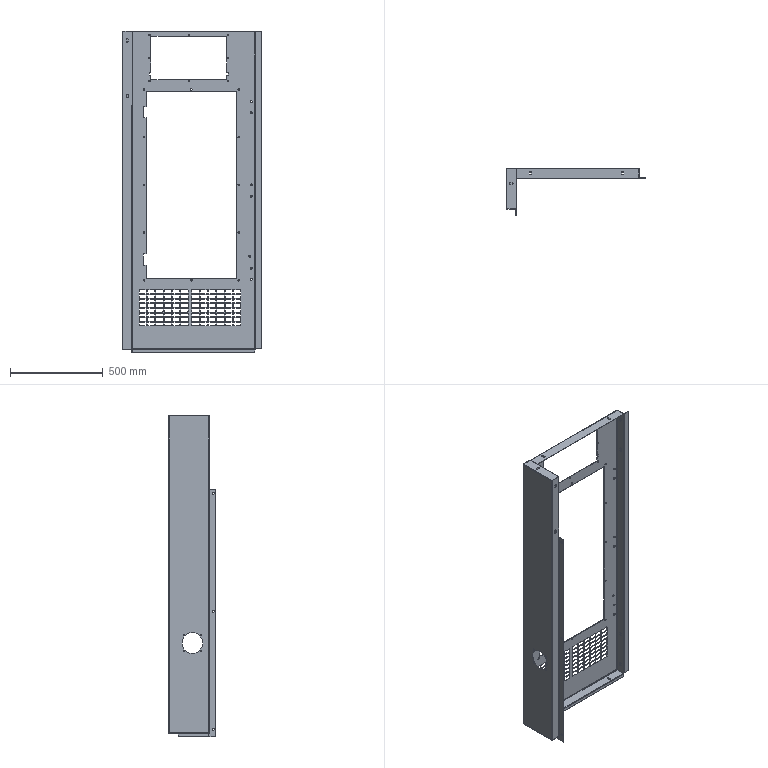Part | STEP file | SYL_0392D6J1SYL0380DJ10-1575320 | 1 solid | 1054 faces | box 755 x 256 x 1738 mm | volume 2626332 mm3 | plane 522 | cylinder 520 | spline 12 | commonest cylinder face diameters 5 x384 8 x51 10 x42 10.5 x18 4 x11 7 x8